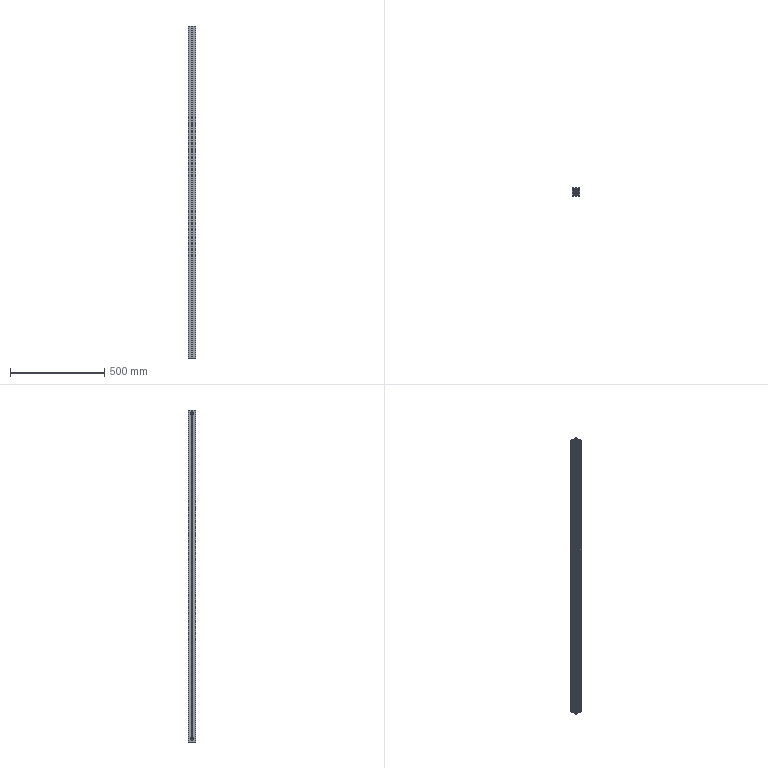Part | SolidWorks | features BaseBody 1, HoleWzd 1, MoveFace 1 | 1 solid | 273 faces | box 40 x 40 x 1762 mm | volume 942816 mm3 | plane 186 | cylinder 87 | commonest cylinder face diameters 0.6 x24 9 x16 10 x16 6.8 x15 2 x8 3 x4